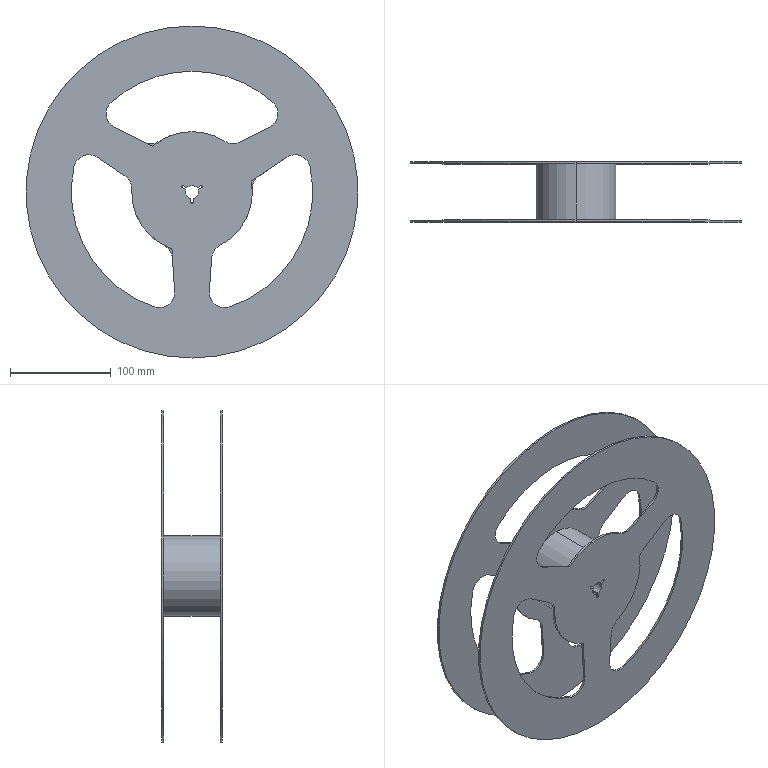Part | STEP file | 11-roller-HSG11 | 1 solid | 78 faces | box 330 x 60 x 330 mm | volume 506877 mm3 | cylinder 56 | plane 22 | commonest cylinder face diameters 30 x25 120 x8 240 x8 2 x5 13 x4 330 x4